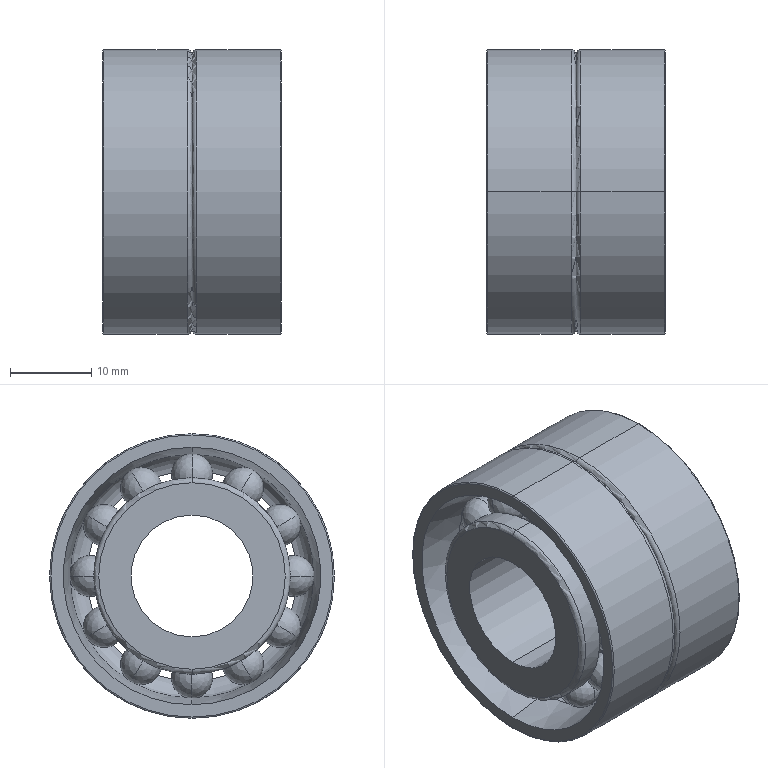Part | NX | features BREP 1 | 1 solid | 202 faces | box 22 x 35 x 35 mm | volume 13233 mm3 | sphere 96 | torus 84 | cylinder 14 | cone 4 | plane 4 | commonest cylinder face diameters 24.132 x6 35 x4 15 x2 25.868 x2